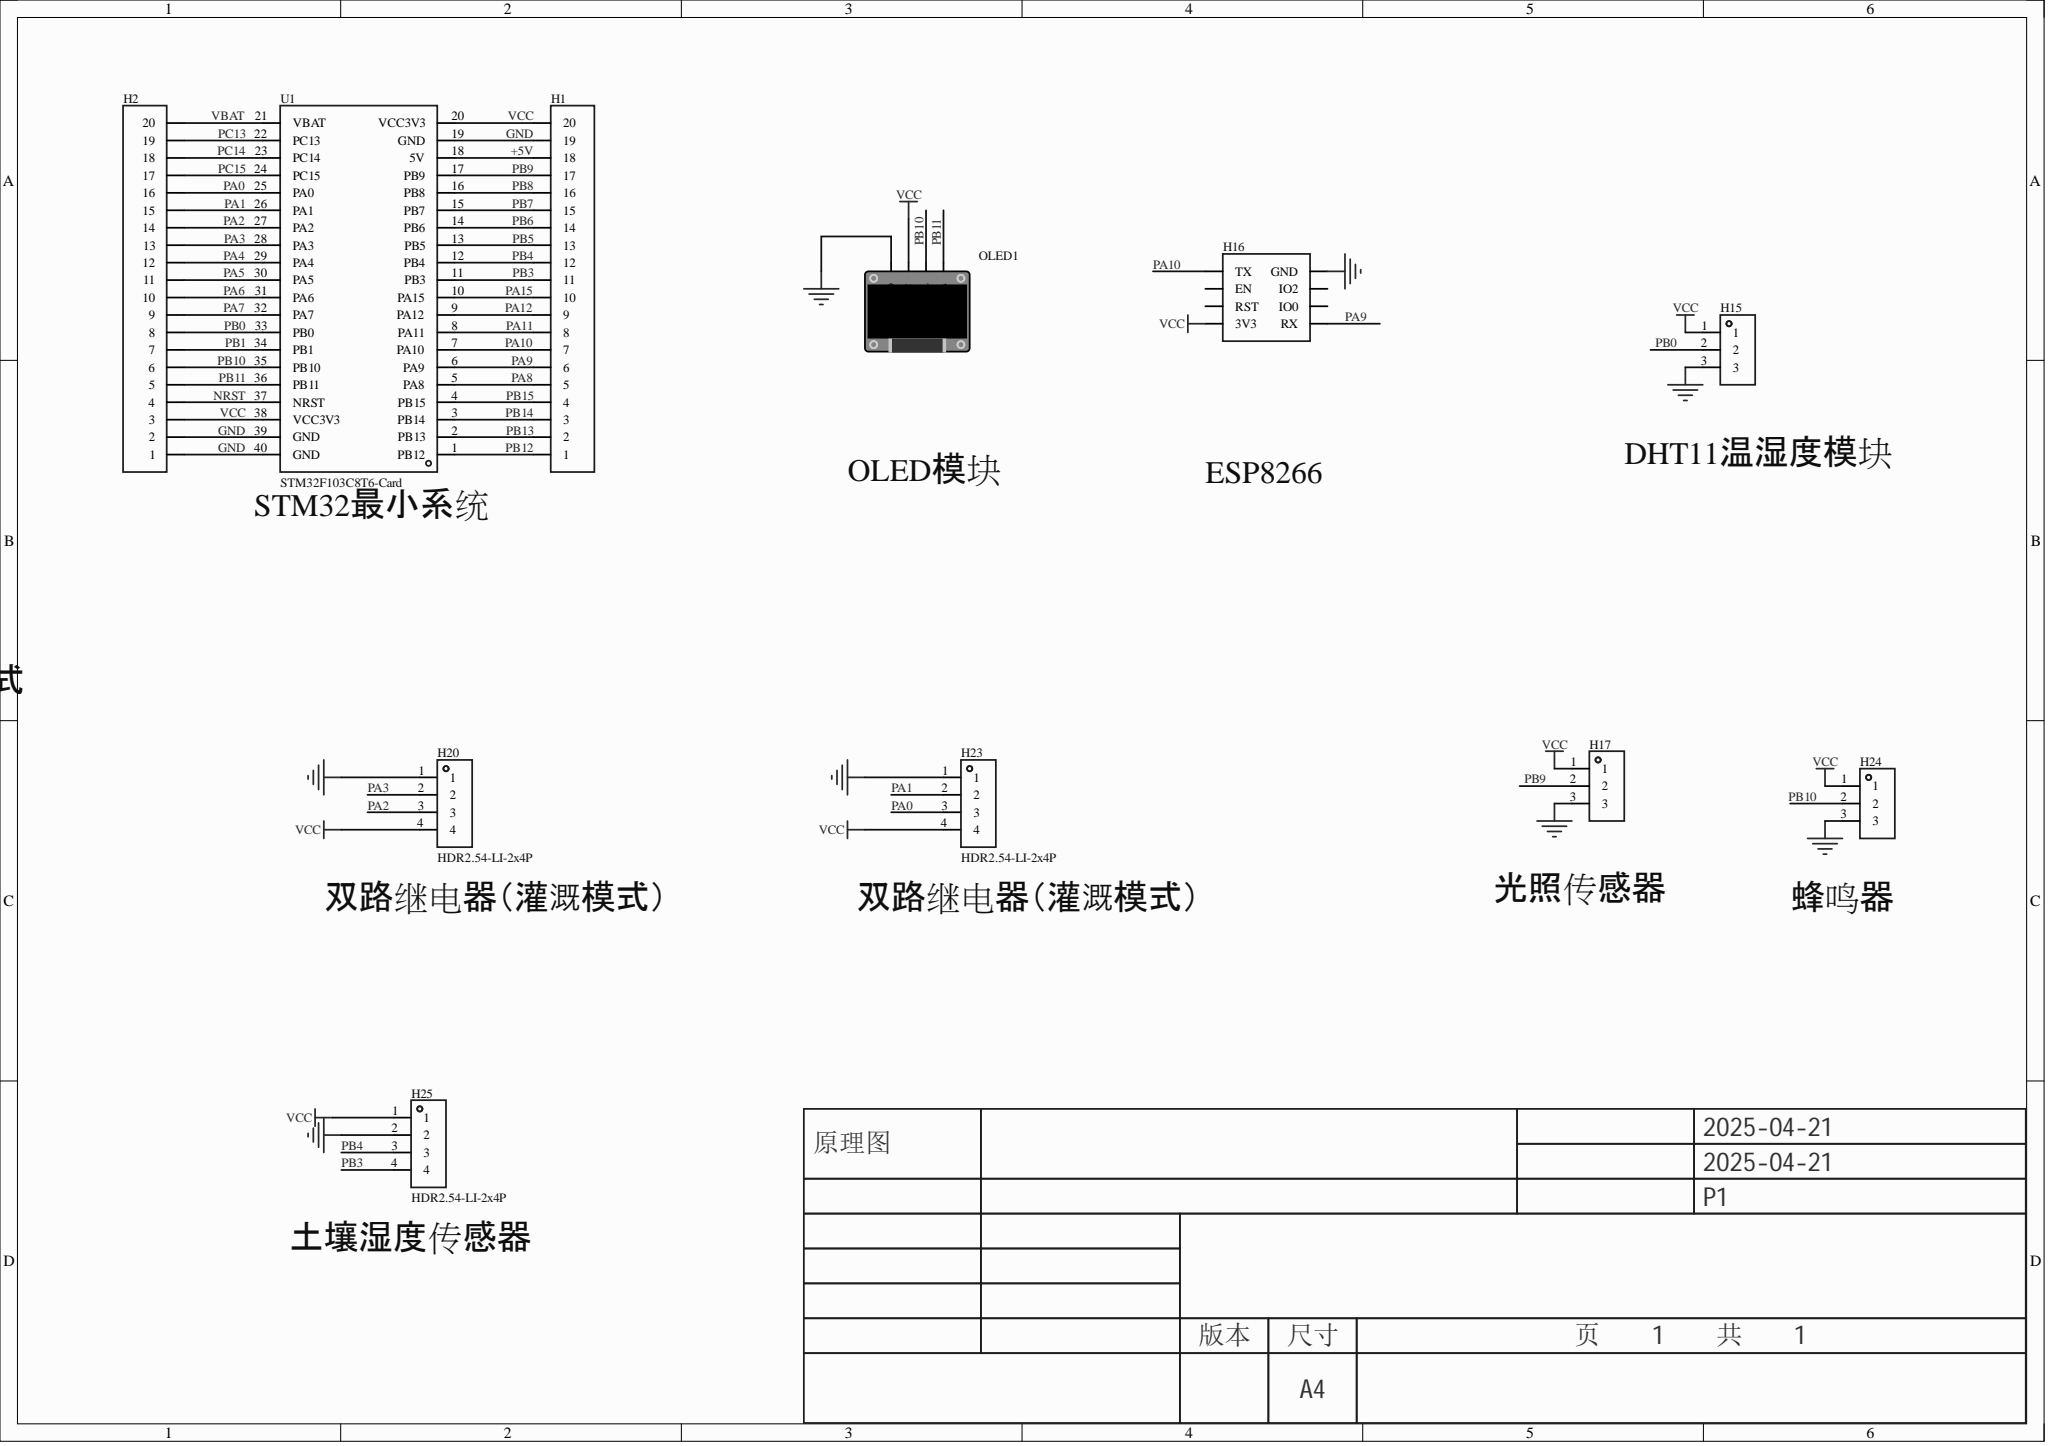Circuit board | Altium Designer | 11 parts | 37 nets
Bill of materials:
Comment,Description,Designator,Footprint,LibRef,Quantity
"","","H1, H2","HDR-TH_20P-P2.54-V-F","HDR-F_2.54_1x20P","2"
"","","H15, H17, H24","HDR-TH_3P-P2.54-V-F","HDR-F_2.54_1x3P","3"
"","","H16","HDR-TH_8P-P2.54-V-F-R2-C4-S2.54-1","HDR-F_2.54_2x4","1"
"HDR2.54-LI-2x4P","","H20, H23, H25","HDR-TH_4P-P2.54-V-M","HDR2.54-LI-2x4P","3"
"","","OLED1","0.96OLED_4P","0.96OLED模块_4P","1"
"STM32F103C8T6-Card","","U1","CONN-TH_L53.3-W22.9_STM32F103C8T6-CARD","STM32F103C8T6-Card","1"
Netlist (Protel format):
[
H1
HDR-TH_20P-P2.54-V-F




]
[
H2
HDR-TH_20P-P2.54-V-F




]
[
H15
HDR-TH_3P-P2.54-V-F




]
[
H16
HDR-TH_8P-P2.54-V-F-R2-C4-S2.54-1




]
[
H17
HDR-TH_3P-P2.54-V-F




]
[
H20
HDR-TH_4P-P2.54-V-M
HDR2.54-LI-2x4P



]
[
H23
HDR-TH_4P-P2.54-V-M
HDR2.54-LI-2x4P



]
[
H24
HDR-TH_3P-P2.54-V-F




]
[
H25
HDR-TH_4P-P2.54-V-M
HDR2.54-LI-2x4P



]
[
OLED1
0.96OLED_4P




]
[
U1
CONN-TH_L53.3-W22.9_STM32F103C8T6-CARD
STM32F103C8T6-Card



]
(
VCC
H1-20
H2-3
H15-1
H16-7
H17-1
H20-4
H23-4
H24-1
H25-1
OLED1-2
U1-20
U1-38
)
(
VBAT
H2-20
U1-21
)
(
PC15
H2-17
U1-24
)
(
PC14
H2-18
U1-23
)
(
PC13
H2-19
U1-22
)
(
PB15
H1-4
U1-4
)
(
PB14
H1-3
U1-3
)
(
PB13
H1-2
U1-2
)
(
PB12
H1-1
U1-1
)
(
PB11
H2-5
OLED1-4
U1-36
)
(
PB10
H2-6
H24-2
OLED1-3
U1-35
)
(
PB9
H1-17
H17-2
U1-17
)
(
PB8
H1-16
U1-16
)
(
PB7
H1-15
U1-15
)
(
PB6
H1-14
U1-14
)
(
PB5
H1-13
U1-13
)
(
PB4
H1-12
H25-3
U1-12
)
(
PB3
H1-11
H25-4
U1-11
)
(
PB1
H2-7
U1-34
)
(
PB0
H2-8
H15-2
U1-33
)
(
PA15
H1-10
U1-10
)
(
PA12
H1-9
U1-9
)
(
PA11
H1-8
U1-8
)
(
PA10
H1-7
H16-1
U1-7
)
(
PA9
H1-6
H16-8
U1-6
)
(
PA8
H1-5
U1-5
)
(
PA7
H2-9
U1-32
)
(
PA6
H2-10
U1-31
)
(
PA5
H2-11
U1-30
)
(
PA4
H2-12
U1-29
)
(
PA3
H2-13
H20-2
U1-28
)
(
PA2
H2-14
H20-3
U1-27
)
(
PA1
H2-15
H23-2
U1-26
)
(
PA0
H2-16
H23-3
U1-25
)
(
NRST
H2-4
U1-37
)
(
GND
H1-19
H2-1
H2-2
H15-3
H16-2
H17-3
H20-1
H23-1
H24-3
H25-2
OLED1-1
U1-19
U1-39
U1-40
)
(
+5V
H1-18
U1-18
)